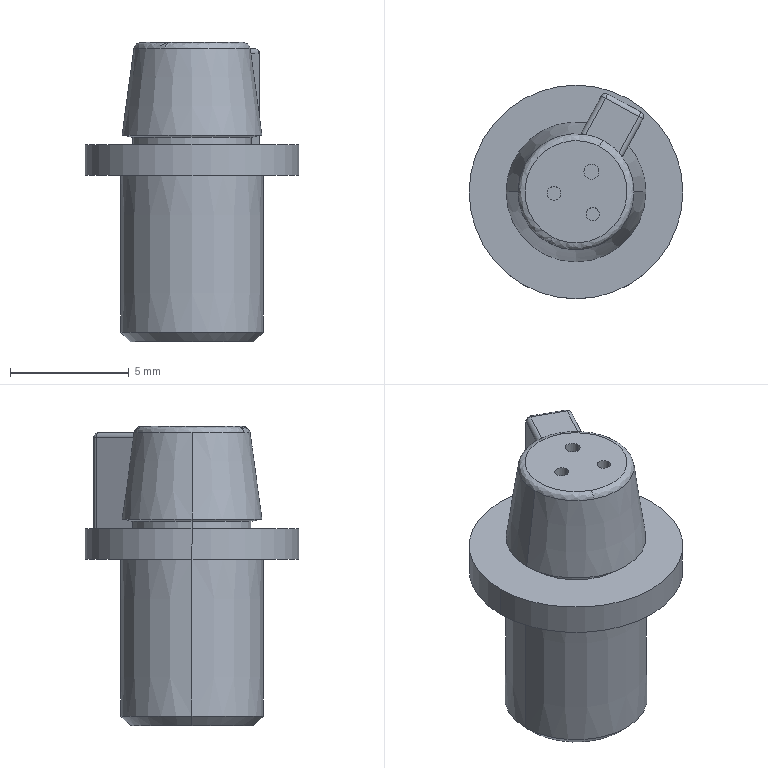Part | SolidWorks | features BaseBody 1 | 1 solid | 45 faces | box 9 x 9 x 12.6 mm | volume 296.292 mm3 | cylinder 19 | plane 12 | cone 10 | spline 4 | commonest cylinder face diameters 0.4 x6 5.005 x3 0.562 x2 0.587 x2 0.63 x2 4 x2
STEP:
#1=CARTESIAN_POINT('',(481.239,-70.69,314.885));
#2=VERTEX_POINT('',#1);
#3=CARTESIAN_POINT('',(480.554,-70.162,314.885));
#4=VERTEX_POINT('',#3);
#5=CARTESIAN_POINT('',(479.428,-72.334,314.885));
#6=DIRECTION('',(0.000000008,-0.000000005,1.));
#7=DIRECTION('',(-1.,0.,0.000000008));
#8=AXIS2_PLACEMENT_3D('',#5,#6,#7);
#9=CIRCLE('',#8,2.447);
#10=EDGE_CURVE('',#2,#4,#9,.T.);
#11=ORIENTED_EDGE('',*,*,#10,.T.);
#12=CARTESIAN_POINT('',(480.417,-70.426,315.144));
#13=VERTEX_POINT('',#12);
#14=CARTESIAN_POINT('',(480.417,-70.426,314.844));
#15=DIRECTION('',(0.8878,-0.4602,-0.000000009));
#16=DIRECTION('',(0.4602,0.8878,0.000000001));
#17=AXIS2_PLACEMENT_3D('',#14,#15,#16);
#18=CIRCLE('',#17,0.3);
#19=EDGE_CURVE('',#4,#13,#18,.T.);
#20=ORIENTED_EDGE('',*,*,#19,.T.);
#21=CARTESIAN_POINT('',(478.438,-74.243,315.144));
#22=VERTEX_POINT('',#21);
#23=CARTESIAN_POINT('',(480.417,-70.426,315.144));
#24=CARTESIAN_POINT('',(484.234,-72.404,315.144));
#25=CARTESIAN_POINT('',(482.255,-76.221,315.144));
#26=CARTESIAN_POINT('',(478.438,-74.243,315.144));
#27=(BOUNDED_CURVE()B_SPLINE_CURVE(3,(#23,#24,#25,#26),.UNSPECIFIED.,.F.,.F.)B_SPLINE_CURVE_WITH_KNOTS((4,4),(0.,1.),.UNSPECIFIED.)CURVE()GEOMETRIC_REPRESENTATION_ITEM()RATIONAL_B_SPLINE_CURVE((1.,0.3333,0.3333,1.))REPRESENTATION_ITEM(''));
#28=EDGE_CURVE('',#13,#22,#27,.T.);
#29=ORIENTED_EDGE('',*,*,#28,.T.);
#30=CARTESIAN_POINT('',(478.302,-74.506,314.885));
#31=VERTEX_POINT('',#30);
#32=CARTESIAN_POINT('',(478.438,-74.243,314.844));
#33=DIRECTION('',(-0.8878,0.4602,0.000000009));
#34=DIRECTION('',(-0.4602,-0.8878,-0.000000001));
#35=AXIS2_PLACEMENT_3D('',#32,#33,#34);
#36=CIRCLE('',#35,0.3);
#37=EDGE_CURVE('',#31,#22,#36,.T.);
#38=ORIENTED_EDGE('',*,*,#37,.F.);
#39=CARTESIAN_POINT('',(481.874,-72.334,314.885));
#40=VERTEX_POINT('',#39);
#41=CARTESIAN_POINT('',(479.428,-72.334,314.885));
#42=DIRECTION('',(-0.000000008,0.000000005,-1.));
#43=DIRECTION('',(0.4602,0.8878,0.000000001));
#44=AXIS2_PLACEMENT_3D('',#41,#42,#43);
#45=CIRCLE('',#44,2.447);
#46=EDGE_CURVE('',#40,#31,#45,.T.);
#47=ORIENTED_EDGE('',*,*,#46,.F.);
#48=CARTESIAN_POINT('',(479.428,-72.334,314.885));
#49=DIRECTION('',(-0.000000008,0.000000005,-1.));
#50=DIRECTION('',(0.4602,0.8878,0.000000001));
#51=AXIS2_PLACEMENT_3D('',#48,#49,#50);
#52=CIRCLE('',#51,2.447);
#53=EDGE_CURVE('',#2,#40,#52,.T.);
#54=ORIENTED_EDGE('',*,*,#53,.F.);
#55=EDGE_LOOP('',(#11,#20,#29,#38,#47,#54));
#56=FACE_OUTER_BOUND('',#55,.T.);
#57=CARTESIAN_POINT('',(480.554,-70.162,314.885));
#58=CARTESIAN_POINT('',(484.898,-72.414,314.885));
#59=CARTESIAN_POINT('',(482.646,-76.759,314.885));
#60=CARTESIAN_POINT('',(478.302,-74.506,314.885));
#61=CARTESIAN_POINT('',(480.544,-70.181,315.041));
#62=CARTESIAN_POINT('',(484.851,-72.413,315.041));
#63=CARTESIAN_POINT('',(482.618,-76.72,315.041));
#64=CARTESIAN_POINT('',(478.311,-74.487,315.041));
#65=CARTESIAN_POINT('',(480.489,-70.286,315.144));
#66=CARTESIAN_POINT('',(484.585,-72.41,315.144));
#67=CARTESIAN_POINT('',(482.462,-76.506,315.144));
#68=CARTESIAN_POINT('',(478.366,-74.382,315.144));
#69=CARTESIAN_POINT('',(480.417,-70.426,315.144));
#70=CARTESIAN_POINT('',(484.234,-72.404,315.144));
#71=CARTESIAN_POINT('',(482.255,-76.221,315.144));
#72=CARTESIAN_POINT('',(478.438,-74.243,315.144));
#73=(BOUNDED_SURFACE()B_SPLINE_SURFACE(3,3,((#57,#58,#59,#60),(#61,#62,#63,#64),(#65,#66,#67,#68),(#69,#70,#71,#72)),.UNSPECIFIED.,.F.,.F.,.F.)B_SPLINE_SURFACE_WITH_KNOTS((4,4),(4,4),(0.,1.),(0.,1.),.UNSPECIFIED.)GEOMETRIC_REPRESENTATION_ITEM()RATIONAL_B_SPLINE_SURFACE(((1.,0.3333,0.3333,1.),(0.8357,0.2786,0.2786,0.8357),(0.8357,0.2786,0.2786,0.8357),(1.,0.3333,0.3333,1.)))REPRESENTATION_ITEM('')SURFACE());
#74=ADVANCED_FACE('',(#56),#73,.T.);
#75=CARTESIAN_POINT('',(482.427,-72.334,302.944));
#76=VERTEX_POINT('',#75);
#77=CARTESIAN_POINT('',(476.429,-72.334,302.944));
#78=VERTEX_POINT('',#77);
#79=CARTESIAN_POINT('',(479.428,-72.334,302.944));
#80=DIRECTION('',(0.000000008,-0.000000005,1.));
#81=DIRECTION('',(0.8773,-0.4799,-0.000000009));
#82=AXIS2_PLACEMENT_3D('',#79,#80,#81);
#83=CIRCLE('',#82,2.999);
#84=EDGE_CURVE('',#76,#78,#83,.T.);
#85=ORIENTED_EDGE('',*,*,#84,.T.);
#86=CARTESIAN_POINT('',(476.428,-72.334,309.544));
#87=VERTEX_POINT('',#86);
#88=CARTESIAN_POINT('',(476.428,-72.334,309.544));
#89=DIRECTION('',(-0.0001745,-0.000000005,1.));
#90=VECTOR('',#89,1000.);
#91=LINE('',#88,#90);
#92=EDGE_CURVE('',#78,#87,#91,.T.);
#93=ORIENTED_EDGE('',*,*,#92,.T.);
#94=CARTESIAN_POINT('',(482.428,-72.334,309.544));
#95=VERTEX_POINT('',#94);
#96=CARTESIAN_POINT('',(479.428,-72.334,309.544));
#97=DIRECTION('',(-0.000000008,0.000000005,-1.));
#98=DIRECTION('',(1.,0.,-0.000000008));
#99=AXIS2_PLACEMENT_3D('',#96,#97,#98);
#100=CIRCLE('',#99,3.);
#101=EDGE_CURVE('',#87,#95,#100,.T.);
#102=ORIENTED_EDGE('',*,*,#101,.T.);
#103=CARTESIAN_POINT('',(482.428,-72.334,309.544));
#104=DIRECTION('',(0.0001745,-0.000000005,1.));
#105=VECTOR('',#104,1000.);
#106=LINE('',#103,#105);
#107=EDGE_CURVE('',#76,#95,#106,.T.);
#108=ORIENTED_EDGE('',*,*,#107,.F.);
#109=EDGE_LOOP('',(#85,#93,#102,#108));
#110=FACE_OUTER_BOUND('',#109,.T.);
#111=CARTESIAN_POINT('',(479.428,-72.334,309.544));
#112=DIRECTION('',(0.000000008,-0.000000005,1.));
#113=DIRECTION('',(1.,0.,-0.000000008));
#114=AXIS2_PLACEMENT_3D('',#111,#112,#113);
#115=CONICAL_SURFACE('',#114,3.,0.0001745);
#116=ADVANCED_FACE('',(#110),#115,.T.);
#117=CARTESIAN_POINT('',(482.026,-72.334,302.544));
#118=VERTEX_POINT('',#117);
#119=CARTESIAN_POINT('',(476.829,-72.334,302.544));
#120=VERTEX_POINT('',#119);
#121=CARTESIAN_POINT('',(479.428,-72.334,302.544));
#122=DIRECTION('',(0.000000008,-0.000000005,1.));
#123=DIRECTION('',(1.,0.,-0.000000008));
#124=AXIS2_PLACEMENT_3D('',#121,#122,#123);
#125=CIRCLE('',#124,2.599);
#126=EDGE_CURVE('',#118,#120,#125,.T.);
#127=ORIENTED_EDGE('',*,*,#126,.T.);
#128=CARTESIAN_POINT('',(476.429,-72.334,302.944));
#129=DIRECTION('',(-0.7072,-0.000000003,0.707));
#130=VECTOR('',#129,1000.);
#131=LINE('',#128,#130);
#132=EDGE_CURVE('',#120,#78,#131,.T.);
#133=ORIENTED_EDGE('',*,*,#132,.T.);
#134=ORIENTED_EDGE('',*,*,#84,.F.);
#135=CARTESIAN_POINT('',(482.427,-72.334,302.944));
#136=DIRECTION('',(0.7072,-0.000000003,0.707));
#137=VECTOR('',#136,1000.);
#138=LINE('',#135,#137);
#139=EDGE_CURVE('',#118,#76,#138,.T.);
#140=ORIENTED_EDGE('',*,*,#139,.F.);
#141=EDGE_LOOP('',(#127,#133,#134,#140));
#142=FACE_OUTER_BOUND('',#141,.T.);
#143=CARTESIAN_POINT('',(479.428,-72.334,302.944));
#144=DIRECTION('',(0.000000008,-0.000000005,1.));
#145=DIRECTION('',(1.,0.,-0.000000008));
#146=AXIS2_PLACEMENT_3D('',#143,#144,#145);
#147=CONICAL_SURFACE('',#146,2.999,0.7855);
#148=ADVANCED_FACE('',(#142),#147,.T.);
#149=CARTESIAN_POINT('',(474.928,-72.334,310.844));
#150=VERTEX_POINT('',#149);
#151=CARTESIAN_POINT('',(483.928,-72.334,310.844));
#152=VERTEX_POINT('',#151);
#153=CARTESIAN_POINT('',(479.428,-72.334,310.844));
#154=DIRECTION('',(-0.000000008,0.000000005,-1.));
#155=DIRECTION('',(-1.,0.,0.000000008));
#156=AXIS2_PLACEMENT_3D('',#153,#154,#155);
#157=CIRCLE('',#156,4.5);
#158=EDGE_CURVE('',#150,#152,#157,.T.);
#159=ORIENTED_EDGE('',*,*,#158,.T.);
#160=CARTESIAN_POINT('',(483.928,-72.334,309.544));
#161=VERTEX_POINT('',#160);
#162=CARTESIAN_POINT('',(483.928,-72.334,309.544));
#163=DIRECTION('',(-0.000000008,0.000000005,-1.));
#164=VECTOR('',#163,1000.);
#165=LINE('',#162,#164);
#166=EDGE_CURVE('',#152,#161,#165,.T.);
#167=ORIENTED_EDGE('',*,*,#166,.T.);
#168=CARTESIAN_POINT('',(474.928,-72.334,309.544));
#169=VERTEX_POINT('',#168);
#170=CARTESIAN_POINT('',(479.428,-72.334,309.544));
#171=DIRECTION('',(0.000000008,-0.000000005,1.));
#172=DIRECTION('',(-1.,0.,0.000000008));
#173=AXIS2_PLACEMENT_3D('',#170,#171,#172);
#174=CIRCLE('',#173,4.5);
#175=EDGE_CURVE('',#161,#169,#174,.T.);
#176=ORIENTED_EDGE('',*,*,#175,.T.);
#177=CARTESIAN_POINT('',(474.928,-72.334,309.544));
#178=DIRECTION('',(-0.000000008,0.000000005,-1.));
#179=VECTOR('',#178,1000.);
#180=LINE('',#177,#179);
#181=EDGE_CURVE('',#150,#169,#180,.T.);
#182=ORIENTED_EDGE('',*,*,#181,.F.);
#183=EDGE_LOOP('',(#159,#167,#176,#182));
#184=FACE_OUTER_BOUND('',#183,.T.);
#185=CARTESIAN_POINT('',(479.428,-72.334,309.544));
#186=DIRECTION('',(-0.000000008,0.000000005,-1.));
#187=DIRECTION('',(-1.,0.,0.000000008));
#188=AXIS2_PLACEMENT_3D('',#185,#186,#187);
#189=CYLINDRICAL_SURFACE('',#188,4.5);
#190=ADVANCED_FACE('',(#184),#189,.T.);
#191=CARTESIAN_POINT('',(481.428,-72.334,309.544));
#192=VERTEX_POINT('',#191);
#193=CARTESIAN_POINT('',(477.428,-72.334,309.544));
#194=VERTEX_POINT('',#193);
#195=CARTESIAN_POINT('',(479.428,-72.334,309.544));
#196=DIRECTION('',(-0.000000008,0.000000005,-1.));
#197=DIRECTION('',(-1.,0.,0.000000008));
#198=AXIS2_PLACEMENT_3D('',#195,#196,#197);
#199=CIRCLE('',#198,2.);
#200=EDGE_CURVE('',#192,#194,#199,.T.);
#201=ORIENTED_EDGE('',*,*,#200,.F.);
#202=CARTESIAN_POINT('',(481.428,-72.334,302.544));
#203=VERTEX_POINT('',#202);
#204=CARTESIAN_POINT('',(481.428,-72.334,302.544));
#205=DIRECTION('',(-0.000000008,0.000000005,-1.));
#206=VECTOR('',#205,1000.);
#207=LINE('',#204,#206);
#208=EDGE_CURVE('',#192,#203,#207,.T.);
#209=ORIENTED_EDGE('',*,*,#208,.T.);
#210=CARTESIAN_POINT('',(477.428,-72.334,302.544));
#211=VERTEX_POINT('',#210);
#212=CARTESIAN_POINT('',(479.428,-72.334,302.544));
#213=DIRECTION('',(0.000000008,-0.000000005,1.));
#214=DIRECTION('',(-1.,0.,0.000000008));
#215=AXIS2_PLACEMENT_3D('',#212,#213,#214);
#216=CIRCLE('',#215,2.);
#217=EDGE_CURVE('',#211,#203,#216,.T.);
#218=ORIENTED_EDGE('',*,*,#217,.F.);
#219=CARTESIAN_POINT('',(477.428,-72.334,302.544));
#220=DIRECTION('',(-0.000000008,0.000000005,-1.));
#221=VECTOR('',#220,1000.);
#222=LINE('',#219,#221);
#223=EDGE_CURVE('',#194,#211,#222,.T.);
#224=ORIENTED_EDGE('',*,*,#223,.F.);
#225=EDGE_LOOP('',(#201,#209,#218,#224));
#226=FACE_OUTER_BOUND('',#225,.T.);
#227=CARTESIAN_POINT('',(479.428,-72.334,302.544));
#228=DIRECTION('',(-0.000000008,0.000000005,-1.));
#229=DIRECTION('',(-1.,0.,0.000000008));
#230=AXIS2_PLACEMENT_3D('',#227,#228,#229);
#231=CYLINDRICAL_SURFACE('',#230,2.);
#232=ADVANCED_FACE('',(#226),#231,.F.);
#233=CARTESIAN_POINT('',(476.925,-72.334,310.844));
#234=VERTEX_POINT('',#233);
#235=CARTESIAN_POINT('',(479.652,-69.842,310.844));
#236=VERTEX_POINT('',#235);
#237=CARTESIAN_POINT('',(479.428,-72.334,310.844));
#238=DIRECTION('',(-0.000000008,0.000000005,-1.));
#239=DIRECTION('',(1.,0.,-0.000000008));
#240=AXIS2_PLACEMENT_3D('',#237,#238,#239);
#241=CIRCLE('',#240,2.503);
#242=EDGE_CURVE('',#234,#236,#241,.T.);
#243=ORIENTED_EDGE('',*,*,#242,.F.);
#244=CARTESIAN_POINT('',(476.925,-72.334,311.148));
#245=VERTEX_POINT('',#244);
#246=CARTESIAN_POINT('',(476.925,-72.334,310.996));
#247=DIRECTION('',(0.000000008,-0.000000005,1.));
#248=VECTOR('',#247,1000.);
#249=LINE('',#246,#248);
#250=EDGE_CURVE('',#234,#245,#249,.T.);
#251=ORIENTED_EDGE('',*,*,#250,.T.);
#252=CARTESIAN_POINT('',(479.652,-69.842,311.148));
#253=VERTEX_POINT('',#252);
#254=CARTESIAN_POINT('',(479.428,-72.334,311.148));
#255=DIRECTION('',(-0.000000008,0.000000005,-1.));
#256=DIRECTION('',(1.,0.,-0.000000008));
#257=AXIS2_PLACEMENT_3D('',#254,#255,#256);
#258=CIRCLE('',#257,2.503);
#259=EDGE_CURVE('',#245,#253,#258,.T.);
#260=ORIENTED_EDGE('',*,*,#259,.T.);
#261=CARTESIAN_POINT('',(479.652,-69.842,310.996));
#262=DIRECTION('',(-0.000000008,0.000000005,-1.));
#263=VECTOR('',#262,1000.);
#264=LINE('',#261,#263);
#265=EDGE_CURVE('',#253,#236,#264,.T.);
#266=ORIENTED_EDGE('',*,*,#265,.T.);
#267=EDGE_LOOP('',(#243,#251,#260,#266));
#268=FACE_OUTER_BOUND('',#267,.T.);
#269=CARTESIAN_POINT('',(479.428,-72.334,310.996));
#270=DIRECTION('',(0.000000008,-0.000000005,1.));
#271=DIRECTION('',(1.,0.,-0.000000008));
#272=AXIS2_PLACEMENT_3D('',#269,#270,#271);
#273=CYLINDRICAL_SURFACE('',#272,2.503);
#274=ADVANCED_FACE('',(#268),#273,.T.);
#275=ORIENTED_EDGE('',*,*,#250,.F.);
#276=CARTESIAN_POINT('',(481.93,-72.334,310.844));
#277=VERTEX_POINT('',#276);
#278=CARTESIAN_POINT('',(479.428,-72.334,310.844));
#279=DIRECTION('',(-0.000000008,0.000000005,-1.));
#280=DIRECTION('',(1.,0.,-0.000000008));
#281=AXIS2_PLACEMENT_3D('',#278,#279,#280);
#282=CIRCLE('',#281,2.503);
#283=EDGE_CURVE('',#277,#234,#282,.T.);
#284=ORIENTED_EDGE('',*,*,#283,.F.);
#285=CARTESIAN_POINT('',(481.93,-72.334,311.148));
#286=VERTEX_POINT('',#285);
#287=CARTESIAN_POINT('',(481.93,-72.334,310.996));
#288=DIRECTION('',(0.000000008,-0.000000005,1.));
#289=VECTOR('',#288,1000.);
#290=LINE('',#287,#289);
#291=EDGE_CURVE('',#277,#286,#290,.T.);
#292=ORIENTED_EDGE('',*,*,#291,.T.);
#293=CARTESIAN_POINT('',(479.428,-72.334,311.148));
#294=DIRECTION('',(-0.000000008,0.000000005,-1.));
#295=DIRECTION('',(1.,0.,-0.000000008));
#296=AXIS2_PLACEMENT_3D('',#293,#294,#295);
#297=CIRCLE('',#296,2.503);
#298=EDGE_CURVE('',#286,#245,#297,.T.);
#299=ORIENTED_EDGE('',*,*,#298,.T.);
#300=EDGE_LOOP('',(#275,#284,#292,#299));
#301=FACE_OUTER_BOUND('',#300,.T.);
#302=CARTESIAN_POINT('',(479.428,-72.334,310.996));
#303=DIRECTION('',(0.000000008,-0.000000005,1.));
#304=DIRECTION('',(1.,0.,-0.000000008));
#305=AXIS2_PLACEMENT_3D('',#302,#303,#304);
#306=CYLINDRICAL_SURFACE('',#305,2.503);
#307=ADVANCED_FACE('',(#301),#306,.T.);
#308=ORIENTED_EDGE('',*,*,#259,.F.);
#309=CARTESIAN_POINT('',(476.482,-72.334,311.244));
#310=VERTEX_POINT('',#309);
#311=CARTESIAN_POINT('',(476.482,-72.334,311.244));
#312=DIRECTION('',(-0.9773,-0.000000001,0.2119));
#313=VECTOR('',#312,1000.);
#314=LINE('',#311,#313);
#315=EDGE_CURVE('',#245,#310,#314,.T.);
#316=ORIENTED_EDGE('',*,*,#315,.T.);
#317=CARTESIAN_POINT('',(479.88,-69.424,311.244));
#318=VERTEX_POINT('',#317);
#319=CARTESIAN_POINT('',(479.428,-72.334,311.244));
#320=DIRECTION('',(-0.000000008,0.000000005,-1.));
#321=DIRECTION('',(0.4602,0.8878,0.000000001));
#322=AXIS2_PLACEMENT_3D('',#319,#320,#321);
#323=CIRCLE('',#322,2.945);
#324=EDGE_CURVE('',#310,#318,#323,.T.);
#325=ORIENTED_EDGE('',*,*,#324,.T.);
#326=CARTESIAN_POINT('',(479.652,-69.842,311.148));
#327=CARTESIAN_POINT('',(479.728,-69.702,311.179));
#328=CARTESIAN_POINT('',(479.804,-69.563,311.211));
#329=CARTESIAN_POINT('',(479.88,-69.424,311.244));
#330=B_SPLINE_CURVE_WITH_KNOTS('',3,(#326,#327,#328,#329),.UNSPECIFIED.,.F.,.F.,(4,4),(0.,0.0004857),.UNSPECIFIED.);
#331=EDGE_CURVE('',#253,#318,#330,.T.);
#332=ORIENTED_EDGE('',*,*,#331,.F.);
#333=EDGE_LOOP('',(#308,#316,#325,#332));
#334=FACE_OUTER_BOUND('',#333,.T.);
#335=CARTESIAN_POINT('',(479.428,-72.334,311.244));
#336=DIRECTION('',(0.000000008,-0.000000005,1.));
#337=DIRECTION('',(1.,0.,-0.000000008));
#338=AXIS2_PLACEMENT_3D('',#335,#336,#337);
#339=CONICAL_SURFACE('',#338,2.945,1.357);
#340=ADVANCED_FACE('',(#334),#339,.T.);
#341=ORIENTED_EDGE('',*,*,#315,.F.);
#342=ORIENTED_EDGE('',*,*,#298,.F.);
#343=CARTESIAN_POINT('',(482.373,-72.334,311.244));
#344=VERTEX_POINT('',#343);
#345=CARTESIAN_POINT('',(482.373,-72.334,311.244));
#346=DIRECTION('',(0.9773,-0.000000001,0.2119));
#347=VECTOR('',#346,1000.);
#348=LINE('',#345,#347);
#349=EDGE_CURVE('',#286,#344,#348,.T.);
#350=ORIENTED_EDGE('',*,*,#349,.T.);
#351=CARTESIAN_POINT('',(479.428,-72.334,311.244));
#352=DIRECTION('',(-0.000000008,0.000000005,-1.));
#353=DIRECTION('',(0.4602,0.8878,0.000000001));
#354=AXIS2_PLACEMENT_3D('',#351,#352,#353);
#355=CIRCLE('',#354,2.945);
#356=EDGE_CURVE('',#344,#310,#355,.T.);
#357=ORIENTED_EDGE('',*,*,#356,.T.);
#358=EDGE_LOOP('',(#341,#342,#350,#357));
#359=FACE_OUTER_BOUND('',#358,.T.);
#360=CARTESIAN_POINT('',(479.428,-72.334,311.244));
#361=DIRECTION('',(0.000000008,-0.000000005,1.));
#362=DIRECTION('',(1.,0.,-0.000000008));
#363=AXIS2_PLACEMENT_3D('',#360,#361,#362);
#364=CONICAL_SURFACE('',#363,2.945,1.357);
#365=ADVANCED_FACE('',(#359),#364,.T.);
#366=CARTESIAN_POINT('',(482.251,-69.257,310.844));
#367=VERTEX_POINT('',#366);
#368=CARTESIAN_POINT('',(482.276,-69.161,310.844));
#369=VERTEX_POINT('',#368);
#370=CARTESIAN_POINT('',(482.076,-69.161,310.844));
#371=DIRECTION('',(0.000000008,-0.000000005,1.));
#372=DIRECTION('',(1.,0.,-0.000000008));
#373=AXIS2_PLACEMENT_3D('',#370,#371,#372);
#374=CIRCLE('',#373,0.2);
#375=EDGE_CURVE('',#367,#369,#374,.T.);
#376=ORIENTED_EDGE('',*,*,#375,.T.);
#377=CARTESIAN_POINT('',(482.276,-69.161,314.685));
#378=VERTEX_POINT('',#377);
#379=CARTESIAN_POINT('',(482.276,-69.161,310.844));
#380=DIRECTION('',(0.000000008,-0.000000005,1.));
#381=VECTOR('',#380,1000.);
#382=LINE('',#379,#381);
#383=EDGE_CURVE('',#369,#378,#382,.T.);
#384=ORIENTED_EDGE('',*,*,#383,.T.);
#385=CARTESIAN_POINT('',(482.251,-69.257,314.685));
#386=VERTEX_POINT('',#385);
#387=CARTESIAN_POINT('',(482.076,-69.161,314.685));
#388=DIRECTION('',(-0.000000008,0.000000005,-1.));
#389=DIRECTION('',(1.,0.,-0.000000008));
#390=AXIS2_PLACEMENT_3D('',#387,#388,#389);
#391=CIRCLE('',#390,0.2);
#392=EDGE_CURVE('',#378,#386,#391,.T.);
#393=ORIENTED_EDGE('',*,*,#392,.T.);
#394=CARTESIAN_POINT('',(482.251,-69.257,310.844));
#395=DIRECTION('',(0.000000008,-0.000000004,1.));
#396=VECTOR('',#395,1000.);
#397=LINE('',#394,#396);
#398=EDGE_CURVE('',#367,#386,#397,.T.);
#399=ORIENTED_EDGE('',*,*,#398,.F.);
#400=EDGE_LOOP('',(#376,#384,#393,#399));
#401=FACE_OUTER_BOUND('',#400,.T.);
#402=CARTESIAN_POINT('',(482.076,-69.161,310.844));
#403=DIRECTION('',(0.000000008,-0.000000005,1.));
#404=DIRECTION('',(1.,0.,-0.000000008));
#405=AXIS2_PLACEMENT_3D('',#402,#403,#404);
#406=CYLINDRICAL_SURFACE('',#405,0.2);
#407=ADVANCED_FACE('',(#401),#406,.T.);
#408=ORIENTED_EDGE('',*,*,#53,.T.);
#409=CARTESIAN_POINT('',(482.373,-72.334,311.244));
#410=DIRECTION('',(0.1356,0.000000005,-0.9908));
#411=VECTOR('',#410,1000.);
#412=LINE('',#409,#411);
#413=EDGE_CURVE('',#40,#344,#412,.T.);
#414=ORIENTED_EDGE('',*,*,#413,.T.);
#415=CARTESIAN_POINT('',(481.635,-70.384,311.244));
#416=VERTEX_POINT('',#415);
#417=CARTESIAN_POINT('',(479.428,-72.334,311.244));
#418=DIRECTION('',(-0.000000008,0.000000005,-1.));
#419=DIRECTION('',(0.4602,0.8878,0.000000001));
#420=AXIS2_PLACEMENT_3D('',#417,#418,#419);
#421=CIRCLE('',#420,2.945);
#422=EDGE_CURVE('',#416,#344,#421,.T.);
#423=ORIENTED_EDGE('',*,*,#422,.F.);
#424=CARTESIAN_POINT('',(481.391,-70.829,314.685));
#425=VERTEX_POINT('',#424);
#426=CARTESIAN_POINT('',(481.391,-70.829,314.685));
#427=CARTESIAN_POINT('',(481.474,-70.678,313.538));
#428=CARTESIAN_POINT('',(481.555,-70.53,312.391));
#429=CARTESIAN_POINT('',(481.635,-70.384,311.244));
#430=B_SPLINE_CURVE_WITH_KNOTS('',3,(#426,#427,#428,#429),.UNSPECIFIED.,.F.,.F.,(4,4),(0.,0.003478),.UNSPECIFIED.);
#431=EDGE_CURVE('',#425,#416,#430,.T.);
#432=ORIENTED_EDGE('',*,*,#431,.F.);
#433=CARTESIAN_POINT('',(481.391,-70.829,314.685));
#434=CARTESIAN_POINT('',(481.387,-70.836,314.738));
#435=CARTESIAN_POINT('',(481.369,-70.823,314.792));
#436=CARTESIAN_POINT('',(481.312,-70.768,314.865));
#437=CARTESIAN_POINT('',(481.276,-70.73,314.885));
#438=CARTESIAN_POINT('',(481.239,-70.69,314.885));
#439=B_SPLINE_CURVE_WITH_KNOTS('',3,(#433,#434,#435,#436,#437,#438),.UNSPECIFIED.,.F.,.F.,(4,2,4),(0.,0.0001598,0.0003197),.UNSPECIFIED.);
#440=EDGE_CURVE('',#425,#2,#439,.T.);
#441=ORIENTED_EDGE('',*,*,#440,.T.);
#442=EDGE_LOOP('',(#408,#414,#423,#432,#441));
#443=FACE_OUTER_BOUND('',#442,.T.);
#444=CARTESIAN_POINT('',(479.428,-72.334,311.244));
#445=DIRECTION('',(-0.000000008,0.000000005,-1.));
#446=DIRECTION('',(-1.,0.,0.000000008));
#447=AXIS2_PLACEMENT_3D('',#444,#445,#446);
#448=CONICAL_SURFACE('',#447,2.945,0.1361);
#449=ADVANCED_FACE('',(#443),#448,.T.);
#450=ORIENTED_EDGE('',*,*,#413,.F.);
#451=ORIENTED_EDGE('',*,*,#46,.T.);
#452=CARTESIAN_POINT('',(476.981,-72.334,314.885));
#453=VERTEX_POINT('',#452);
#454=CARTESIAN_POINT('',(479.428,-72.334,314.885));
#455=DIRECTION('',(-0.000000008,0.000000005,-1.));
#456=DIRECTION('',(0.4602,0.8878,0.000000001));
#457=AXIS2_PLACEMENT_3D('',#454,#455,#456);
#458=CIRCLE('',#457,2.447);
#459=EDGE_CURVE('',#31,#453,#458,.T.);
#460=ORIENTED_EDGE('',*,*,#459,.T.);
#461=CARTESIAN_POINT('',(476.482,-72.334,311.244));
#462=DIRECTION('',(-0.1356,0.000000005,-0.9908));
#463=VECTOR('',#462,1000.);
#464=LINE('',#461,#463);
#465=EDGE_CURVE('',#453,#310,#464,.T.);
#466=ORIENTED_EDGE('',*,*,#465,.T.);
#467=ORIENTED_EDGE('',*,*,#356,.F.);
#468=EDGE_LOOP('',(#450,#451,#460,#466,#467));
#469=FACE_OUTER_BOUND('',#468,.T.);
#470=CARTESIAN_POINT('',(479.428,-72.334,311.244));
#471=DIRECTION('',(-0.000000008,0.000000005,-1.));
#472=DIRECTION('',(-1.,0.,0.000000008));
#473=AXIS2_PLACEMENT_3D('',#470,#471,#472);
#474=CONICAL_SURFACE('',#473,2.945,0.1361);
#475=ADVANCED_FACE('',(#469),#474,.T.);
#476=CARTESIAN_POINT('',(479.762,-71.484,310.144));
#477=VERTEX_POINT('',#476);
#478=CARTESIAN_POINT('',(480.392,-71.484,310.144));
#479=VERTEX_POINT('',#478);
#480=CARTESIAN_POINT('',(480.077,-71.484,310.144));
#481=DIRECTION('',(0.000000008,-0.000000005,1.));
#482=DIRECTION('',(1.,0.,-0.000000008));
#483=AXIS2_PLACEMENT_3D('',#480,#481,#482);
#484=CIRCLE('',#483,0.3151);
#485=EDGE_CURVE('',#477,#479,#484,.T.);
#486=ORIENTED_EDGE('',*,*,#485,.F.);
#487=CARTESIAN_POINT('',(479.762,-71.484,315.144));
#488=VERTEX_POINT('',#487);
#489=CARTESIAN_POINT('',(479.762,-71.484,315.144));
#490=DIRECTION('',(0.000000008,-0.000000005,1.));
#491=VECTOR('',#490,1000.);
#492=LINE('',#489,#491);
#493=EDGE_CURVE('',#477,#488,#492,.T.);
#494=ORIENTED_EDGE('',*,*,#493,.T.);
#495=CARTESIAN_POINT('',(480.392,-71.484,315.144));
#496=VERTEX_POINT('',#495);
#497=CARTESIAN_POINT('',(480.077,-71.484,315.144));
#498=DIRECTION('',(-0.000000008,0.000000005,-1.));
#499=DIRECTION('',(1.,0.,-0.000000008));
#500=AXIS2_PLACEMENT_3D('',#497,#498,#499);
#501=CIRCLE('',#500,0.3151);
#502=EDGE_CURVE('',#496,#488,#501,.T.);
#503=ORIENTED_EDGE('',*,*,#502,.F.);
#504=CARTESIAN_POINT('',(480.392,-71.484,315.144));
#505=DIRECTION('',(0.000000008,-0.000000005,1.));
#506=VECTOR('',#505,1000.);
#507=LINE('',#504,#506);
#508=EDGE_CURVE('',#479,#496,#507,.T.);
#509=ORIENTED_EDGE('',*,*,#508,.F.);
#510=EDGE_LOOP('',(#486,#494,#503,#509));
#511=FACE_OUTER_BOUND('',#510,.T.);
#512=CARTESIAN_POINT('',(480.077,-71.484,315.144));
#513=DIRECTION('',(0.000000008,-0.000000005,1.));
#514=DIRECTION('',(1.,0.,-0.000000008));
#515=AXIS2_PLACEMENT_3D('',#512,#513,#514);
#516=CYLINDRICAL_SURFACE('',#515,0.3151);
#517=ADVANCED_FACE('',(#511),#516,.F.);
#518=CARTESIAN_POINT('',(479.856,-73.279,310.144));
#519=VERTEX_POINT('',#518);
#520=CARTESIAN_POINT('',(480.418,-73.279,310.144));
#521=VERTEX_POINT('',#520);
#522=CARTESIAN_POINT('',(480.137,-73.279,310.144));
#523=DIRECTION('',(0.000000008,-0.000000005,1.));
#524=DIRECTION('',(1.,0.,-0.000000008));
#525=AXIS2_PLACEMENT_3D('',#522,#523,#524);
#526=CIRCLE('',#525,0.2808);
#527=EDGE_CURVE('',#519,#521,#526,.T.);
#528=ORIENTED_EDGE('',*,*,#527,.F.);
#529=CARTESIAN_POINT('',(479.856,-73.279,315.144));
#530=VERTEX_POINT('',#529);
#531=CARTESIAN_POINT('',(479.856,-73.279,315.144));
#532=DIRECTION('',(0.000000008,-0.000000005,1.));
#533=VECTOR('',#532,1000.);
#534=LINE('',#531,#533);
#535=EDGE_CURVE('',#519,#530,#534,.T.);
#536=ORIENTED_EDGE('',*,*,#535,.T.);
#537=CARTESIAN_POINT('',(480.418,-73.279,315.144));
#538=VERTEX_POINT('',#537);
#539=CARTESIAN_POINT('',(480.137,-73.279,315.144));
#540=DIRECTION('',(-0.000000008,0.000000005,-1.));
#541=DIRECTION('',(1.,0.,-0.000000008));
#542=AXIS2_PLACEMENT_3D('',#539,#540,#541);
#543=CIRCLE('',#542,0.2808);
#544=EDGE_CURVE('',#538,#530,#543,.T.);
#545=ORIENTED_EDGE('',*,*,#544,.F.);
#546=CARTESIAN_POINT('',(480.418,-73.279,315.144));
#547=DIRECTION('',(0.000000008,-0.000000005,1.));
#548=VECTOR('',#547,1000.);
#549=LINE('',#546,#548);
#550=EDGE_CURVE('',#521,#538,#549,.T.);
#551=ORIENTED_EDGE('',*,*,#550,.F.);
#552=EDGE_LOOP('',(#528,#536,#545,#551));
#553=FACE_OUTER_BOUND('',#552,.T.);
#554=CARTESIAN_POINT('',(480.137,-73.279,315.144));
#555=DIRECTION('',(0.000000008,-0.000000005,1.));
#556=DIRECTION('',(1.,0.,-0.000000008));
#557=AXIS2_PLACEMENT_3D('',#554,#555,#556);
#558=CYLINDRICAL_SURFACE('',#557,0.2808);
#559=ADVANCED_FACE('',(#553),#558,.F.);
#560=CARTESIAN_POINT('',(478.209,-72.4,310.144));
#561=VERTEX_POINT('',#560);
#562=CARTESIAN_POINT('',(478.795,-72.4,310.144));
#563=VERTEX_POINT('',#562);
#564=CARTESIAN_POINT('',(478.502,-72.4,310.144));
#565=DIRECTION('',(0.000000008,-0.000000005,1.));
#566=DIRECTION('',(1.,0.,-0.000000008));
#567=AXIS2_PLACEMENT_3D('',#564,#565,#566);
#568=CIRCLE('',#567,0.2933);
#569=EDGE_CURVE('',#561,#563,#568,.T.);
#570=ORIENTED_EDGE('',*,*,#569,.F.);
#571=CARTESIAN_POINT('',(478.209,-72.4,315.144));
#572=VERTEX_POINT('',#571);
#573=CARTESIAN_POINT('',(478.209,-72.4,315.144));
#574=DIRECTION('',(0.000000008,-0.000000005,1.));
#575=VECTOR('',#574,1000.);
#576=LINE('',#573,#575);
#577=EDGE_CURVE('',#561,#572,#576,.T.);
#578=ORIENTED_EDGE('',*,*,#577,.T.);
#579=CARTESIAN_POINT('',(478.795,-72.4,315.144));
#580=VERTEX_POINT('',#579);
#581=CARTESIAN_POINT('',(478.502,-72.4,315.144));
#582=DIRECTION('',(-0.000000008,0.000000005,-1.));
#583=DIRECTION('',(1.,0.,-0.000000008));
#584=AXIS2_PLACEMENT_3D('',#581,#582,#583);
#585=CIRCLE('',#584,0.2933);
#586=EDGE_CURVE('',#580,#572,#585,.T.);
#587=ORIENTED_EDGE('',*,*,#586,.F.);
#588=CARTESIAN_POINT('',(478.795,-72.4,315.144));
#589=DIRECTION('',(0.000000008,-0.000000005,1.));
#590=VECTOR('',#589,1000.);
#591=LINE('',#588,#590);
#592=EDGE_CURVE('',#563,#580,#591,.T.);
#593=ORIENTED_EDGE('',*,*,#592,.F.);
#594=EDGE_LOOP('',(#570,#578,#587,#593));
#595=FACE_OUTER_BOUND('',#594,.T.);
#596=CARTESIAN_POINT('',(478.502,-72.4,315.144));
#597=DIRECTION('',(0.000000008,-0.000000005,1.));
#598=DIRECTION('',(1.,0.,-0.000000008));
#599=AXIS2_PLACEMENT_3D('',#596,#597,#598);
#600=CYLINDRICAL_SURFACE('',#599,0.2933);
#601=ADVANCED_FACE('',(#595),#600,.F.);
#602=ORIENTED_EDGE('',*,*,#92,.F.);
#603=CARTESIAN_POINT('',(479.428,-72.334,302.944));
#604=DIRECTION('',(0.000000008,-0.000000005,1.));
#605=DIRECTION('',(0.8773,-0.4799,-0.000000009));
#606=AXIS2_PLACEMENT_3D('',#603,#604,#605);
#607=CIRCLE('',#606,2.999);
#608=EDGE_CURVE('',#78,#76,#607,.T.);
#609=ORIENTED_EDGE('',*,*,#608,.T.);
#610=ORIENTED_EDGE('',*,*,#107,.T.);
#611=CARTESIAN_POINT('',(479.428,-72.334,309.544));
#612=DIRECTION('',(-0.000000008,0.000000005,-1.));
#613=DIRECTION('',(1.,0.,-0.000000008));
#614=AXIS2_PLACEMENT_3D('',#611,#612,#613);
#615=CIRCLE('',#614,3.);
#616=EDGE_CURVE('',#95,#87,#615,.T.);
#617=ORIENTED_EDGE('',*,*,#616,.T.);
#618=EDGE_LOOP('',(#602,#609,#610,#617));
#619=FACE_OUTER_BOUND('',#618,.T.);
#620=CARTESIAN_POINT('',(479.428,-72.334,309.544));
#621=DIRECTION('',(0.000000008,-0.000000005,1.));
#622=DIRECTION('',(1.,0.,-0.000000008));
#623=AXIS2_PLACEMENT_3D('',#620,#621,#622);
#624=CONICAL_SURFACE('',#623,3.,0.0001745);
#625=ADVANCED_FACE('',(#619),#624,.T.);
#626=ORIENTED_EDGE('',*,*,#132,.F.);
#627=CARTESIAN_POINT('',(479.428,-72.334,302.544));
#628=DIRECTION('',(0.000000008,-0.000000005,1.));
#629=DIRECTION('',(1.,0.,-0.000000008));
#630=AXIS2_PLACEMENT_3D('',#627,#628,#629);
#631=CIRCLE('',#630,2.599);
#632=EDGE_CURVE('',#120,#118,#631,.T.);
#633=ORIENTED_EDGE('',*,*,#632,.T.);
#634=ORIENTED_EDGE('',*,*,#139,.T.);
#635=ORIENTED_EDGE('',*,*,#608,.F.);
#636=EDGE_LOOP('',(#626,#633,#634,#635));
#637=FACE_OUTER_BOUND('',#636,.T.);
#638=CARTESIAN_POINT('',(479.428,-72.334,302.944));
#639=DIRECTION('',(0.000000008,-0.000000005,1.));
#640=DIRECTION('',(1.,0.,-0.000000008));
#641=AXIS2_PLACEMENT_3D('',#638,#639,#640);
#642=CONICAL_SURFACE('',#641,2.999,0.7855);
#643=ADVANCED_FACE('',(#637),#642,.T.);
#644=CARTESIAN_POINT('',(479.428,-72.334,309.544));
#645=DIRECTION('',(0.000000008,-0.000000005,1.));
#646=DIRECTION('',(-1.,0.,0.000000008));
#647=AXIS2_PLACEMENT_3D('',#644,#645,#646);
#648=CIRCLE('',#647,4.5);
#649=EDGE_CURVE('',#169,#161,#648,.T.);
#650=ORIENTED_EDGE('',*,*,#649,.F.);
#651=ORIENTED_EDGE('',*,*,#175,.F.);
#652=EDGE_LOOP('',(#650,#651));
#653=FACE_OUTER_BOUND('',#652,.T.);
#654=ORIENTED_EDGE('',*,*,#616,.F.);
#655=ORIENTED_EDGE('',*,*,#101,.F.);
#656=EDGE_LOOP('',(#654,#655));
#657=FACE_BOUND('',#656,.T.);
#658=CARTESIAN_POINT('',(479.428,-72.334,309.544));
#659=DIRECTION('',(0.000000008,-0.000000005,1.));
#660=DIRECTION('',(1.,0.,-0.000000008));
#661=AXIS2_PLACEMENT_3D('',#658,#659,#660);
#662=PLANE('',#661);
#663=ADVANCED_FACE('',(#653,#657),#662,.F.);
#664=ORIENTED_EDGE('',*,*,#126,.F.);
#665=ORIENTED_EDGE('',*,*,#632,.F.);
#666=EDGE_LOOP('',(#664,#665));
#667=FACE_OUTER_BOUND('',#666,.T.);
#668=ORIENTED_EDGE('',*,*,#217,.T.);
#669=CARTESIAN_POINT('',(479.428,-72.334,302.544));
#670=DIRECTION('',(0.000000008,-0.000000005,1.));
#671=DIRECTION('',(-1.,0.,0.000000008));
#672=AXIS2_PLACEMENT_3D('',#669,#670,#671);
#673=CIRCLE('',#672,2.);
#674=EDGE_CURVE('',#203,#211,#673,.T.);
#675=ORIENTED_EDGE('',*,*,#674,.T.);
#676=EDGE_LOOP('',(#668,#675));
#677=FACE_BOUND('',#676,.T.);
#678=CARTESIAN_POINT('',(479.428,-72.334,302.544));
#679=DIRECTION('',(-0.000000008,0.000000005,-1.));
#680=DIRECTION('',(-1.,0.,0.000000008));
#681=AXIS2_PLACEMENT_3D('',#678,#679,#680);
#682=PLANE('',#681);
#683=ADVANCED_FACE('',(#667,#677),#682,.T.);
#684=ORIENTED_EDGE('',*,*,#166,.F.);
#685=CARTESIAN_POINT('',(479.428,-72.334,310.844));
#686=DIRECTION('',(-0.000000008,0.000000005,-1.));
#687=DIRECTION('',(-1.,0.,0.000000008));
#688=AXIS2_PLACEMENT_3D('',#685,#686,#687);
#689=CIRCLE('',#688,4.5);
#690=EDGE_CURVE('',#152,#150,#689,.T.);
#691=ORIENTED_EDGE('',*,*,#690,.T.);
#692=ORIENTED_EDGE('',*,*,#181,.T.);
#693=ORIENTED_EDGE('',*,*,#649,.T.);
#694=EDGE_LOOP('',(#684,#691,#692,#693));
#695=FACE_OUTER_BOUND('',#694,.T.);
#696=CARTESIAN_POINT('',(479.428,-72.334,309.544));
#697=DIRECTION('',(-0.000000008,0.000000005,-1.));
#698=DIRECTION('',(-1.,0.,0.000000008));
#699=AXIS2_PLACEMENT_3D('',#696,#697,#698);
#700=CYLINDRICAL_SURFACE('',#699,4.5);
#701=ADVANCED_FACE('',(#695),#700,.T.);
#702=ORIENTED_EDGE('',*,*,#208,.F.);
#703=CARTESIAN_POINT('',(479.428,-72.334,309.544));
#704=DIRECTION('',(-0.000000008,0.000000005,-1.));
#705=DIRECTION('',(-1.,0.,0.000000008));
#706=AXIS2_PLACEMENT_3D('',#703,#704,#705);
#707=CIRCLE('',#706,2.);
#708=EDGE_CURVE('',#194,#192,#707,.T.);
#709=ORIENTED_EDGE('',*,*,#708,.F.);
#710=ORIENTED_EDGE('',*,*,#223,.T.);
#711=ORIENTED_EDGE('',*,*,#674,.F.);
#712=EDGE_LOOP('',(#702,#709,#710,#711));
#713=FACE_OUTER_BOUND('',#712,.T.);
#714=CARTESIAN_POINT('',(479.428,-72.334,302.544));
#715=DIRECTION('',(-0.000000008,0.000000005,-1.));
#716=DIRECTION('',(-1.,0.,0.000000008));
#717=AXIS2_PLACEMENT_3D('',#714,#715,#716);
#718=CYLINDRICAL_SURFACE('',#717,2.);
#719=ADVANCED_FACE('',(#713),#718,.F.);
#720=CARTESIAN_POINT('',(481.406,-70.802,310.844));
#721=VERTEX_POINT('',#720);
#722=CARTESIAN_POINT('',(482.251,-69.257,310.844));
#723=DIRECTION('',(-0.4799,-0.8773,0.));
#724=VECTOR('',#723,1000.);
#725=LINE('',#722,#724);
#726=EDGE_CURVE('',#367,#721,#725,.T.);
#727=ORIENTED_EDGE('',*,*,#726,.T.);
#728=CARTESIAN_POINT('',(479.428,-72.334,310.844));
#729=DIRECTION('',(-0.000000008,0.000000005,-1.));
#730=DIRECTION('',(1.,0.,-0.000000008));
#731=AXIS2_PLACEMENT_3D('',#728,#729,#730);
#732=CIRCLE('',#731,2.503);
#733=EDGE_CURVE('',#721,#277,#732,.T.);
#734=ORIENTED_EDGE('',*,*,#733,.T.);
#735=ORIENTED_EDGE('',*,*,#283,.T.);
#736=ORIENTED_EDGE('',*,*,#242,.T.);
#737=CARTESIAN_POINT('',(480.497,-68.297,310.844));
#738=VERTEX_POINT('',#737);
#739=CARTESIAN_POINT('',(479.652,-69.842,310.844));
#740=DIRECTION('',(0.4799,0.8773,0.));
#741=VECTOR('',#740,1000.);
#742=LINE('',#739,#741);
#743=EDGE_CURVE('',#236,#738,#742,.T.);
#744=ORIENTED_EDGE('',*,*,#743,.T.);
#745=CARTESIAN_POINT('',(480.768,-68.217,310.844));
#746=VERTEX_POINT('',#745);
#747=CARTESIAN_POINT('',(480.672,-68.393,310.844));
#748=DIRECTION('',(0.000000008,-0.000000005,1.));
#749=DIRECTION('',(1.,0.,-0.000000008));
#750=AXIS2_PLACEMENT_3D('',#747,#748,#749);
#751=CIRCLE('',#750,0.2);
#752=EDGE_CURVE('',#746,#738,#751,.T.);
#753=ORIENTED_EDGE('',*,*,#752,.F.);
#754=CARTESIAN_POINT('',(482.172,-68.985,310.844));
#755=VERTEX_POINT('',#754);
#756=CARTESIAN_POINT('',(480.593,-68.121,310.844));
#757=DIRECTION('',(-0.8773,0.4799,0.));
#758=VECTOR('',#757,1000.);
#759=LINE('',#756,#758);
#760=EDGE_CURVE('',#755,#746,#759,.T.);
#761=ORIENTED_EDGE('',*,*,#760,.F.);
#762=CARTESIAN_POINT('',(482.076,-69.161,310.844));
#763=DIRECTION('',(0.000000008,-0.000000005,1.));
#764=DIRECTION('',(1.,0.,-0.000000008));
#765=AXIS2_PLACEMENT_3D('',#762,#763,#764);
#766=CIRCLE('',#765,0.2);
#767=EDGE_CURVE('',#369,#755,#766,.T.);
#768=ORIENTED_EDGE('',*,*,#767,.F.);
#769=ORIENTED_EDGE('',*,*,#375,.F.);
#770=EDGE_LOOP('',(#727,#734,#735,#736,#744,#753,#761,#768,#769));
#771=FACE_BOUND('',#770,.T.);
#772=ORIENTED_EDGE('',*,*,#158,.F.);
#773=ORIENTED_EDGE('',*,*,#690,.F.);
#774=EDGE_LOOP('',(#772,#773));
#775=FACE_OUTER_BOUND('',#774,.T.);
#776=CARTESIAN_POINT('',(479.428,-72.334,310.844));
#777=DIRECTION('',(0.000000008,-0.000000005,1.));
#778=DIRECTION('',(1.,0.,-0.000000008));
#779=AXIS2_PLACEMENT_3D('',#776,#777,#778);
#780=PLANE('',#779);
#781=ADVANCED_FACE('',(#771,#775),#780,.T.);
#782=ORIENTED_EDGE('',*,*,#708,.T.);
#783=ORIENTED_EDGE('',*,*,#200,.T.);
#784=EDGE_LOOP('',(#782,#783));
#785=FACE_OUTER_BOUND('',#784,.T.);
#786=CARTESIAN_POINT('',(479.428,-72.334,309.544));
#787=DIRECTION('',(0.000000008,-0.000000005,1.));
#788=DIRECTION('',(1.,0.,-0.000000008));
#789=AXIS2_PLACEMENT_3D('',#786,#787,#788);
#790=PLANE('',#789);
#791=ADVANCED_FACE('',(#785),#790,.F.);
#792=ORIENTED_EDGE('',*,*,#291,.F.);
#793=ORIENTED_EDGE('',*,*,#733,.F.);
#794=CARTESIAN_POINT('',(481.406,-70.802,311.148));
#795=VERTEX_POINT('',#794);
#796=CARTESIAN_POINT('',(481.406,-70.802,310.996));
#797=DIRECTION('',(0.000000008,-0.000000005,1.));
#798=VECTOR('',#797,1000.);
#799=LINE('',#796,#798);
#800=EDGE_CURVE('',#721,#795,#799,.T.);
#801=ORIENTED_EDGE('',*,*,#800,.T.);
#802=CARTESIAN_POINT('',(479.428,-72.334,311.148));
#803=DIRECTION('',(-0.000000008,0.000000005,-1.));
#804=DIRECTION('',(1.,0.,-0.000000008));
#805=AXIS2_PLACEMENT_3D('',#802,#803,#804);
#806=CIRCLE('',#805,2.503);
#807=EDGE_CURVE('',#795,#286,#806,.T.);
#808=ORIENTED_EDGE('',*,*,#807,.T.);
#809=EDGE_LOOP('',(#792,#793,#801,#808));
#810=FACE_OUTER_BOUND('',#809,.T.);
#811=CARTESIAN_POINT('',(479.428,-72.334,310.996));
#812=DIRECTION('',(0.000000008,-0.000000005,1.));
#813=DIRECTION('',(1.,0.,-0.000000008));
#814=AXIS2_PLACEMENT_3D('',#811,#812,#813);
#815=CYLINDRICAL_SURFACE('',#814,2.503);
#816=ADVANCED_FACE('',(#810),#815,.T.);
#817=ORIENTED_EDGE('',*,*,#726,.F.);
#818=ORIENTED_EDGE('',*,*,#398,.T.);
#819=CARTESIAN_POINT('',(482.347,-69.081,314.685));
#820=DIRECTION('',(-0.4799,-0.8773,0.));
#821=VECTOR('',#820,1000.);
#822=LINE('',#819,#821);
#823=EDGE_CURVE('',#386,#425,#822,.T.);
#824=ORIENTED_EDGE('',*,*,#823,.T.);
#825=ORIENTED_EDGE('',*,*,#431,.T.);
#826=CARTESIAN_POINT('',(481.635,-70.384,311.244));
#827=CARTESIAN_POINT('',(481.559,-70.523,311.211));
#828=CARTESIAN_POINT('',(481.482,-70.662,311.179));
#829=CARTESIAN_POINT('',(481.406,-70.802,311.148));
#830=B_SPLINE_CURVE_WITH_KNOTS('',3,(#826,#827,#828,#829),.UNSPECIFIED.,.F.,.F.,(4,4),(0.,0.0004857),.UNSPECIFIED.);
#831=EDGE_CURVE('',#416,#795,#830,.T.);
#832=ORIENTED_EDGE('',*,*,#831,.T.);
#833=ORIENTED_EDGE('',*,*,#800,.F.);
#834=EDGE_LOOP('',(#817,#818,#824,#825,#832,#833));
#835=FACE_OUTER_BOUND('',#834,.T.);
#836=CARTESIAN_POINT('',(482.347,-69.081,310.844));
#837=DIRECTION('',(0.8773,-0.4799,-0.000000009));
#838=DIRECTION('',(0.4799,0.8773,0.));
#839=AXIS2_PLACEMENT_3D('',#836,#837,#838);
#840=PLANE('',#839);
#841=ADVANCED_FACE('',(#835),#840,.T.);
#842=ORIENTED_EDGE('',*,*,#331,.T.);
#843=CARTESIAN_POINT('',(479.637,-69.869,314.685));
#844=VERTEX_POINT('',#843);
#845=CARTESIAN_POINT('',(479.88,-69.424,311.244));
#846=CARTESIAN_POINT('',(479.8,-69.57,312.391));
#847=CARTESIAN_POINT('',(479.719,-69.718,313.538));
#848=CARTESIAN_POINT('',(479.637,-69.869,314.685));
#849=B_SPLINE_CURVE_WITH_KNOTS('',3,(#845,#846,#847,#848),.UNSPECIFIED.,.F.,.F.,(4,4),(0.,0.003478),.UNSPECIFIED.);
#850=EDGE_CURVE('',#318,#844,#849,.T.);
#851=ORIENTED_EDGE('',*,*,#850,.T.);
#852=CARTESIAN_POINT('',(480.497,-68.297,314.685));
#853=VERTEX_POINT('',#852);
#854=CARTESIAN_POINT('',(479.537,-70.052,314.685));
#855=DIRECTION('',(0.4799,0.8773,0.));
#856=VECTOR('',#855,1000.);
#857=LINE('',#854,#856);
#858=EDGE_CURVE('',#844,#853,#857,.T.);
#859=ORIENTED_EDGE('',*,*,#858,.T.);
#860=CARTESIAN_POINT('',(480.497,-68.297,310.844));
#861=DIRECTION('',(-0.000000008,0.000000004,-1.));
#862=VECTOR('',#861,1000.);
#863=LINE('',#860,#862);
#864=EDGE_CURVE('',#853,#738,#863,.T.);
#865=ORIENTED_EDGE('',*,*,#864,.T.);
#866=ORIENTED_EDGE('',*,*,#743,.F.);
#867=ORIENTED_EDGE('',*,*,#265,.F.);
#868=EDGE_LOOP('',(#842,#851,#859,#865,#866,#867));
#869=FACE_OUTER_BOUND('',#868,.T.);
#870=CARTESIAN_POINT('',(479.537,-70.052,310.844));
#871=DIRECTION('',(-0.8773,0.4799,0.000000009));
#872=DIRECTION('',(-0.4799,-0.8773,0.));
#873=AXIS2_PLACEMENT_3D('',#870,#871,#872);
#874=PLANE('',#873);
#875=ADVANCED_FACE('',(#869),#874,.T.);
#876=ORIENTED_EDGE('',*,*,#349,.F.);
#877=ORIENTED_EDGE('',*,*,#807,.F.);
#878=ORIENTED_EDGE('',*,*,#831,.F.);
#879=ORIENTED_EDGE('',*,*,#422,.T.);
#880=EDGE_LOOP('',(#876,#877,#878,#879));
#881=FACE_OUTER_BOUND('',#880,.T.);
#882=CARTESIAN_POINT('',(479.428,-72.334,311.244));
#883=DIRECTION('',(0.000000008,-0.000000005,1.));
#884=DIRECTION('',(1.,0.,-0.000000008));
#885=AXIS2_PLACEMENT_3D('',#882,#883,#884);
#886=CONICAL_SURFACE('',#885,2.945,1.357);
#887=ADVANCED_FACE('',(#881),#886,.T.);
#888=ORIENTED_EDGE('',*,*,#383,.F.);
#889=ORIENTED_EDGE('',*,*,#767,.T.);
#890=CARTESIAN_POINT('',(482.172,-68.985,314.685));
#891=VERTEX_POINT('',#890);
#892=CARTESIAN_POINT('',(482.172,-68.985,310.844));
#893=DIRECTION('',(0.000000008,-0.000000005,1.));
#894=VECTOR('',#893,1000.);
#895=LINE('',#892,#894);
#896=EDGE_CURVE('',#755,#891,#895,.T.);
#897=ORIENTED_EDGE('',*,*,#896,.T.);
#898=CARTESIAN_POINT('',(482.076,-69.161,314.685));
#899=DIRECTION('',(-0.000000008,0.000000005,-1.));
#900=DIRECTION('',(1.,0.,-0.000000008));
#901=AXIS2_PLACEMENT_3D('',#898,#899,#900);
#902=CIRCLE('',#901,0.2);
#903=EDGE_CURVE('',#891,#378,#902,.T.);
#904=ORIENTED_EDGE('',*,*,#903,.T.);
#905=EDGE_LOOP('',(#888,#889,#897,#904));
#906=FACE_OUTER_BOUND('',#905,.T.);
#907=CARTESIAN_POINT('',(482.076,-69.161,310.844));
#908=DIRECTION('',(0.000000008,-0.000000005,1.));
#909=DIRECTION('',(1.,0.,-0.000000008));
#910=AXIS2_PLACEMENT_3D('',#907,#908,#909);
#911=CYLINDRICAL_SURFACE('',#910,0.2);
#912=ADVANCED_FACE('',(#906),#911,.T.);
#913=ORIENTED_EDGE('',*,*,#465,.F.);
#914=CARTESIAN_POINT('',(479.836,-69.922,314.885));
#915=VERTEX_POINT('',#914);
#916=CARTESIAN_POINT('',(479.428,-72.334,314.885));
#917=DIRECTION('',(-0.000000008,0.000000005,-1.));
#918=DIRECTION('',(0.4602,0.8878,0.000000001));
#919=AXIS2_PLACEMENT_3D('',#916,#917,#918);
#920=CIRCLE('',#919,2.447);
#921=EDGE_CURVE('',#453,#915,#920,.T.);
#922=ORIENTED_EDGE('',*,*,#921,.T.);
#923=CARTESIAN_POINT('',(479.836,-69.922,314.885));
#924=CARTESIAN_POINT('',(479.783,-69.913,314.885));
#925=CARTESIAN_POINT('',(479.73,-69.903,314.865));
#926=CARTESIAN_POINT('',(479.654,-69.885,314.792));
#927=CARTESIAN_POINT('',(479.633,-69.876,314.738));
#928=CARTESIAN_POINT('',(479.637,-69.869,314.685));
#929=B_SPLINE_CURVE_WITH_KNOTS('',3,(#923,#924,#925,#926,#927,#928),.UNSPECIFIED.,.F.,.F.,(4,2,4),(-0.000163,-0.000002991,0.000157),.UNSPECIFIED.);
#930=EDGE_CURVE('',#915,#844,#929,.T.);
#931=ORIENTED_EDGE('',*,*,#930,.T.);
#932=ORIENTED_EDGE('',*,*,#850,.F.);
#933=ORIENTED_EDGE('',*,*,#324,.F.);
#934=EDGE_LOOP('',(#913,#922,#931,#932,#933));
#935=FACE_OUTER_BOUND('',#934,.T.);
#936=CARTESIAN_POINT('',(479.428,-72.334,311.244));
#937=DIRECTION('',(-0.000000008,0.000000005,-1.));
#938=DIRECTION('',(-1.,0.,0.000000008));
#939=AXIS2_PLACEMENT_3D('',#936,#937,#938);
#940=CONICAL_SURFACE('',#939,2.945,0.1361);
#941=ADVANCED_FACE('',(#935),#940,.T.);
#942=ORIENTED_EDGE('',*,*,#823,.F.);
#943=CARTESIAN_POINT('',(482.076,-69.161,314.885));
#944=VERTEX_POINT('',#943);
#945=CARTESIAN_POINT('',(482.076,-69.161,314.685));
#946=DIRECTION('',(-0.4799,-0.8773,0.));
#947=DIRECTION('',(0.8773,-0.4799,0.));
#948=AXIS2_PLACEMENT_3D('',#945,#946,#947);
#949=CIRCLE('',#948,0.2);
#950=EDGE_CURVE('',#386,#944,#949,.T.);
#951=ORIENTED_EDGE('',*,*,#950,.T.);
#952=CARTESIAN_POINT('',(481.908,-69.468,314.885));
#953=DIRECTION('',(-0.4799,-0.8773,0.));
#954=VECTOR('',#953,1000.);
#955=LINE('',#952,#954);
#956=EDGE_CURVE('',#944,#2,#955,.T.);
#957=ORIENTED_EDGE('',*,*,#956,.T.);
#958=ORIENTED_EDGE('',*,*,#440,.F.);
#959=EDGE_LOOP('',(#942,#951,#957,#958));
#960=FACE_OUTER_BOUND('',#959,.T.);
#961=CARTESIAN_POINT('',(481.908,-69.468,314.685));
#962=DIRECTION('',(-0.4799,-0.8773,0.));
#963=DIRECTION('',(0.8773,-0.4799,0.));
#964=AXIS2_PLACEMENT_3D('',#961,#962,#963);
#965=CYLINDRICAL_SURFACE('',#964,0.2);
#966=ADVANCED_FACE('',(#960),#965,.T.);
#967=ORIENTED_EDGE('',*,*,#864,.F.);
#968=CARTESIAN_POINT('',(480.768,-68.217,314.685));
#969=VERTEX_POINT('',#968);
#970=CARTESIAN_POINT('',(480.672,-68.393,314.685));
#971=DIRECTION('',(-0.000000008,0.000000005,-1.));
#972=DIRECTION('',(1.,0.,-0.000000008));
#973=AXIS2_PLACEMENT_3D('',#970,#971,#972);
#974=CIRCLE('',#973,0.2);
#975=EDGE_CURVE('',#853,#969,#974,.T.);
#976=ORIENTED_EDGE('',*,*,#975,.T.);
#977=CARTESIAN_POINT('',(480.768,-68.217,310.844));
#978=DIRECTION('',(-0.000000008,0.000000005,-1.));
#979=VECTOR('',#978,1000.);
#980=LINE('',#977,#979);
#981=EDGE_CURVE('',#969,#746,#980,.T.);
#982=ORIENTED_EDGE('',*,*,#981,.T.);
#983=ORIENTED_EDGE('',*,*,#752,.T.);
#984=EDGE_LOOP('',(#967,#976,#982,#983));
#985=FACE_OUTER_BOUND('',#984,.T.);
#986=CARTESIAN_POINT('',(480.672,-68.393,310.844));
#987=DIRECTION('',(0.000000008,-0.000000005,1.));
#988=DIRECTION('',(1.,0.,-0.000000008));
#989=AXIS2_PLACEMENT_3D('',#986,#987,#988);
#990=CYLINDRICAL_SURFACE('',#989,0.2);
#991=ADVANCED_FACE('',(#985),#990,.T.);
#992=ORIENTED_EDGE('',*,*,#858,.F.);
#993=ORIENTED_EDGE('',*,*,#930,.F.);
#994=CARTESIAN_POINT('',(480.672,-68.393,314.885));
#995=VERTEX_POINT('',#994);
#996=CARTESIAN_POINT('',(479.976,-69.665,314.885));
#997=DIRECTION('',(0.4799,0.8773,0.));
#998=VECTOR('',#997,1000.);
#999=LINE('',#996,#998);
#1000=EDGE_CURVE('',#915,#995,#999,.T.);
#1001=ORIENTED_EDGE('',*,*,#1000,.T.);
#1002=CARTESIAN_POINT('',(480.672,-68.393,314.685));
#1003=DIRECTION('',(-0.4799,-0.8773,0.));
#1004=DIRECTION('',(-0.8773,0.4799,0.));
#1005=AXIS2_PLACEMENT_3D('',#1002,#1003,#1004);
#1006=CIRCLE('',#1005,0.2);
#1007=EDGE_CURVE('',#995,#853,#1006,.T.);
#1008=ORIENTED_EDGE('',*,*,#1007,.T.);
#1009=EDGE_LOOP('',(#992,#993,#1001,#1008));
#1010=FACE_OUTER_BOUND('',#1009,.T.);
#1011=CARTESIAN_POINT('',(479.976,-69.665,314.685));
#1012=DIRECTION('',(0.4799,0.8773,0.));
#1013=DIRECTION('',(-0.8773,0.4799,0.));
#1014=AXIS2_PLACEMENT_3D('',#1011,#1012,#1013);
#1015=CYLINDRICAL_SURFACE('',#1014,0.2);
#1016=ADVANCED_FACE('',(#1010),#1015,.T.);
#1017=CARTESIAN_POINT('',(482.076,-69.161,314.685));
#1018=DIRECTION('',(-0.8773,0.4799,0.000000009));
#1019=DIRECTION('',(0.4799,0.8773,0.));
#1020=AXIS2_PLACEMENT_3D('',#1017,#1018,#1019);
#1021=CIRCLE('',#1020,0.2);
#1022=EDGE_CURVE('',#944,#891,#1021,.T.);
#1023=ORIENTED_EDGE('',*,*,#1022,.F.);
#1024=ORIENTED_EDGE('',*,*,#950,.F.);
#1025=ORIENTED_EDGE('',*,*,#392,.F.);
#1026=ORIENTED_EDGE('',*,*,#903,.F.);
#1027=EDGE_LOOP('',(#1023,#1024,#1025,#1026));
#1028=FACE_OUTER_BOUND('',#1027,.T.);
#1029=CARTESIAN_POINT('',(482.251,-69.257,314.685));
#1030=CARTESIAN_POINT('',(482.251,-69.257,314.685));
#1031=CARTESIAN_POINT('',(482.251,-69.257,314.685));
#1032=CARTESIAN_POINT('',(482.251,-69.257,314.685));
#1033=CARTESIAN_POINT('',(482.307,-69.154,314.684));
#1034=CARTESIAN_POINT('',(482.308,-69.153,314.753));
#1035=CARTESIAN_POINT('',(482.284,-69.196,314.803));
#1036=CARTESIAN_POINT('',(482.251,-69.258,314.802));
#1037=CARTESIAN_POINT('',(482.275,-69.041,314.683));
#1038=CARTESIAN_POINT('',(482.275,-69.04,314.802));
#1039=CARTESIAN_POINT('',(482.235,-69.114,314.886));
#1040=CARTESIAN_POINT('',(482.178,-69.219,314.885));
#1041=CARTESIAN_POINT('',(482.172,-68.985,314.683));
#1042=CARTESIAN_POINT('',(482.172,-68.984,314.802));
#1043=CARTESIAN_POINT('',(482.132,-69.058,314.886));
#1044=CARTESIAN_POINT('',(482.075,-69.162,314.885));
#1045=(BOUNDED_SURFACE()B_SPLINE_SURFACE(3,3,((#1029,#1030,#1031,#1032),(#1033,#1034,#1035,#1036),(#1037,#1038,#1039,#1040),(#1041,#1042,#1043,#1044)),.UNSPECIFIED.,.F.,.F.,.F.)B_SPLINE_SURFACE_WITH_KNOTS((4,4),(4,4),(0.,1.),(0.,1.),.UNSPECIFIED.)GEOMETRIC_REPRESENTATION_ITEM()RATIONAL_B_SPLINE_SURFACE(((1.,0.8003,0.8003,1.),(0.8047,0.644,0.644,0.8047),(0.8047,0.644,0.644,0.8047),(1.,0.8003,0.8003,1.)))REPRESENTATION_ITEM('')SURFACE());
#1046=ADVANCED_FACE('',(#1028),#1045,.T.);
#1047=ORIENTED_EDGE('',*,*,#19,.F.);
#1048=CARTESIAN_POINT('',(479.428,-72.334,314.885));
#1049=DIRECTION('',(0.000000008,-0.000000005,1.));
#1050=DIRECTION('',(-1.,0.,0.000000008));
#1051=AXIS2_PLACEMENT_3D('',#1048,#1049,#1050);
#1052=CIRCLE('',#1051,2.447);
#1053=EDGE_CURVE('',#4,#915,#1052,.T.);
#1054=ORIENTED_EDGE('',*,*,#1053,.T.);
#1055=ORIENTED_EDGE('',*,*,#921,.F.);
#1056=ORIENTED_EDGE('',*,*,#459,.F.);
#1057=ORIENTED_EDGE('',*,*,#37,.T.);
#1058=CARTESIAN_POINT('',(478.438,-74.243,315.144));
#1059=CARTESIAN_POINT('',(474.622,-72.264,315.144));
#1060=CARTESIAN_POINT('',(476.6,-68.447,315.144));
#1061=CARTESIAN_POINT('',(480.417,-70.426,315.144));
#1062=(BOUNDED_CURVE()B_SPLINE_CURVE(3,(#1058,#1059,#1060,#1061),.UNSPECIFIED.,.F.,.F.)B_SPLINE_CURVE_WITH_KNOTS((4,4),(0.,1.),.UNSPECIFIED.)CURVE()GEOMETRIC_REPRESENTATION_ITEM()RATIONAL_B_SPLINE_CURVE((1.,0.3333,0.3333,1.))REPRESENTATION_ITEM(''));
#1063=EDGE_CURVE('',#22,#13,#1062,.T.);
#1064=ORIENTED_EDGE('',*,*,#1063,.T.);
#1065=EDGE_LOOP('',(#1047,#1054,#1055,#1056,#1057,#1064));
#1066=FACE_OUTER_BOUND('',#1065,.T.);
#1067=CARTESIAN_POINT('',(478.302,-74.506,314.885));
#1068=CARTESIAN_POINT('',(473.957,-72.254,314.885));
#1069=CARTESIAN_POINT('',(476.209,-67.91,314.885));
#1070=CARTESIAN_POINT('',(480.554,-70.162,314.885));
#1071=CARTESIAN_POINT('',(478.311,-74.487,315.041));
#1072=CARTESIAN_POINT('',(474.005,-72.255,315.041));
#1073=CARTESIAN_POINT('',(476.237,-67.948,315.041));
#1074=CARTESIAN_POINT('',(480.544,-70.181,315.041));
#1075=CARTESIAN_POINT('',(478.366,-74.382,315.144));
#1076=CARTESIAN_POINT('',(474.27,-72.259,315.144));
#1077=CARTESIAN_POINT('',(476.393,-68.163,315.144));
#1078=CARTESIAN_POINT('',(480.489,-70.286,315.144));
#1079=CARTESIAN_POINT('',(478.438,-74.243,315.144));
#1080=CARTESIAN_POINT('',(474.622,-72.264,315.144));
#1081=CARTESIAN_POINT('',(476.6,-68.447,315.144));
#1082=CARTESIAN_POINT('',(480.417,-70.426,315.144));
#1083=(BOUNDED_SURFACE()B_SPLINE_SURFACE(3,3,((#1067,#1068,#1069,#1070),(#1071,#1072,#1073,#1074),(#1075,#1076,#1077,#1078),(#1079,#1080,#1081,#1082)),.UNSPECIFIED.,.F.,.F.,.F.)B_SPLINE_SURFACE_WITH_KNOTS((4,4),(4,4),(0.,1.),(0.,1.),.UNSPECIFIED.)GEOMETRIC_REPRESENTATION_ITEM()RATIONAL_B_SPLINE_SURFACE(((1.,0.3333,0.3333,1.),(0.8357,0.2786,0.2786,0.8357),(0.8357,0.2786,0.2786,0.8357),(1.,0.3333,0.3333,1.)))REPRESENTATION_ITEM('')SURFACE());
#1084=ADVANCED_FACE('',(#1066),#1083,.T.);
#1085=CARTESIAN_POINT('',(480.672,-68.393,314.685));
#1086=DIRECTION('',(0.8773,-0.4799,-0.000000009));
#1087=DIRECTION('',(0.4799,0.8773,0.));
#1088=AXIS2_PLACEMENT_3D('',#1085,#1086,#1087);
#1089=CIRCLE('',#1088,0.2);
#1090=EDGE_CURVE('',#969,#995,#1089,.T.);
#1091=ORIENTED_EDGE('',*,*,#1090,.F.);
#1092=ORIENTED_EDGE('',*,*,#975,.F.);
#1093=ORIENTED_EDGE('',*,*,#1007,.F.);
#1094=EDGE_LOOP('',(#1091,#1092,#1093));
#1095=FACE_OUTER_BOUND('',#1094,.T.);
#1096=CARTESIAN_POINT('',(480.77,-68.218,314.685));
#1097=CARTESIAN_POINT('',(480.77,-68.218,314.802));
#1098=CARTESIAN_POINT('',(480.73,-68.291,314.885));
#1099=CARTESIAN_POINT('',(480.674,-68.394,314.885));
#1100=CARTESIAN_POINT('',(480.667,-68.161,314.685));
#1101=CARTESIAN_POINT('',(480.667,-68.161,314.803));
#1102=CARTESIAN_POINT('',(480.627,-68.234,314.886));
#1103=CARTESIAN_POINT('',(480.57,-68.337,314.886));
#1104=CARTESIAN_POINT('',(480.553,-68.193,314.685));
#1105=CARTESIAN_POINT('',(480.553,-68.193,314.754));
#1106=CARTESIAN_POINT('',(480.53,-68.236,314.803));
#1107=CARTESIAN_POINT('',(480.497,-68.297,314.803));
#1108=CARTESIAN_POINT('',(480.497,-68.297,314.685));
#1109=CARTESIAN_POINT('',(480.497,-68.297,314.685));
#1110=CARTESIAN_POINT('',(480.497,-68.297,314.685));
#1111=CARTESIAN_POINT('',(480.497,-68.297,314.685));
#1112=(BOUNDED_SURFACE()B_SPLINE_SURFACE(3,3,((#1096,#1097,#1098,#1099),(#1100,#1101,#1102,#1103),(#1104,#1105,#1106,#1107),(#1108,#1109,#1110,#1111)),.UNSPECIFIED.,.F.,.F.,.F.)B_SPLINE_SURFACE_WITH_KNOTS((4,4),(4,4),(0.,1.),(0.,1.),.UNSPECIFIED.)GEOMETRIC_REPRESENTATION_ITEM()RATIONAL_B_SPLINE_SURFACE(((1.,0.8047,0.8047,1.),(0.8025,0.6458,0.6458,0.8025),(0.8025,0.6458,0.6458,0.8025),(1.,0.8047,0.8047,1.)))REPRESENTATION_ITEM('')SURFACE());
#1113=ADVANCED_FACE('',(#1095),#1112,.T.);
#1114=ORIENTED_EDGE('',*,*,#896,.F.);
#1115=ORIENTED_EDGE('',*,*,#760,.T.);
#1116=ORIENTED_EDGE('',*,*,#981,.F.);
#1117=CARTESIAN_POINT('',(480.593,-68.121,314.685));
#1118=DIRECTION('',(0.8773,-0.4799,0.));
#1119=VECTOR('',#1118,1000.);
#1120=LINE('',#1117,#1119);
#1121=EDGE_CURVE('',#969,#891,#1120,.T.);
#1122=ORIENTED_EDGE('',*,*,#1121,.T.);
#1123=EDGE_LOOP('',(#1114,#1115,#1116,#1122));
#1124=FACE_OUTER_BOUND('',#1123,.T.);
#1125=CARTESIAN_POINT('',(480.593,-68.121,310.844));
#1126=DIRECTION('',(0.4799,0.8773,0.));
#1127=DIRECTION('',(-0.8773,0.4799,0.));
#1128=AXIS2_PLACEMENT_3D('',#1125,#1126,#1127);
#1129=PLANE('',#1128);
#1130=ADVANCED_FACE('',(#1124),#1129,.T.);
#1131=ORIENTED_EDGE('',*,*,#28,.F.);
#1132=ORIENTED_EDGE('',*,*,#1063,.F.);
#1133=EDGE_LOOP('',(#1131,#1132));
#1134=FACE_OUTER_BOUND('',#1133,.T.);
#1135=ORIENTED_EDGE('',*,*,#502,.T.);
#1136=CARTESIAN_POINT('',(480.077,-71.484,315.144));
#1137=DIRECTION('',(-0.000000008,0.000000005,-1.));
#1138=DIRECTION('',(1.,0.,-0.000000008));
#1139=AXIS2_PLACEMENT_3D('',#1136,#1137,#1138);
#1140=CIRCLE('',#1139,0.3151);
#1141=EDGE_CURVE('',#488,#496,#1140,.T.);
#1142=ORIENTED_EDGE('',*,*,#1141,.T.);
#1143=EDGE_LOOP('',(#1135,#1142));
#1144=FACE_BOUND('',#1143,.T.);
#1145=ORIENTED_EDGE('',*,*,#544,.T.);
#1146=CARTESIAN_POINT('',(480.137,-73.279,315.144));
#1147=DIRECTION('',(-0.000000008,0.000000005,-1.));
#1148=DIRECTION('',(1.,0.,-0.000000008));
#1149=AXIS2_PLACEMENT_3D('',#1146,#1147,#1148);
#1150=CIRCLE('',#1149,0.2808);
#1151=EDGE_CURVE('',#530,#538,#1150,.T.);
#1152=ORIENTED_EDGE('',*,*,#1151,.T.);
#1153=EDGE_LOOP('',(#1145,#1152));
#1154=FACE_BOUND('',#1153,.T.);
#1155=ORIENTED_EDGE('',*,*,#586,.T.);
#1156=CARTESIAN_POINT('',(478.502,-72.4,315.144));
#1157=DIRECTION('',(-0.000000008,0.000000005,-1.));
#1158=DIRECTION('',(1.,0.,-0.000000008));
#1159=AXIS2_PLACEMENT_3D('',#1156,#1157,#1158);
#1160=CIRCLE('',#1159,0.2933);
#1161=EDGE_CURVE('',#572,#580,#1160,.T.);
#1162=ORIENTED_EDGE('',*,*,#1161,.T.);
#1163=EDGE_LOOP('',(#1155,#1162));
#1164=FACE_BOUND('',#1163,.T.);
#1165=CARTESIAN_POINT('',(479.983,-71.264,315.144));
#1166=DIRECTION('',(0.000000008,-0.000000005,1.));
#1167=DIRECTION('',(1.,0.,-0.000000008));
#1168=AXIS2_PLACEMENT_3D('',#1165,#1166,#1167);
#1169=PLANE('',#1168);
#1170=ADVANCED_FACE('',(#1134,#1144,#1154,#1164),#1169,.T.);
#1171=ORIENTED_EDGE('',*,*,#956,.F.);
#1172=CARTESIAN_POINT('',(482.076,-69.161,314.885));
#1173=DIRECTION('',(-0.8773,0.4799,0.000000009));
#1174=VECTOR('',#1173,1000.);
#1175=LINE('',#1172,#1174);
#1176=EDGE_CURVE('',#944,#995,#1175,.T.);
#1177=ORIENTED_EDGE('',*,*,#1176,.T.);
#1178=ORIENTED_EDGE('',*,*,#1000,.F.);
#1179=ORIENTED_EDGE('',*,*,#1053,.F.);
#1180=ORIENTED_EDGE('',*,*,#10,.F.);
#1181=EDGE_LOOP('',(#1171,#1177,#1178,#1179,#1180));
#1182=FACE_OUTER_BOUND('',#1181,.T.);
#1183=CARTESIAN_POINT('',(480.942,-69.566,314.885));
#1184=DIRECTION('',(0.000000008,-0.000000005,1.));
#1185=DIRECTION('',(1.,0.,-0.000000008));
#1186=AXIS2_PLACEMENT_3D('',#1183,#1184,#1185);
#1187=PLANE('',#1186);
#1188=ADVANCED_FACE('',(#1182),#1187,.T.);
#1189=ORIENTED_EDGE('',*,*,#1121,.F.);
#1190=ORIENTED_EDGE('',*,*,#1090,.T.);
#1191=ORIENTED_EDGE('',*,*,#1176,.F.);
#1192=ORIENTED_EDGE('',*,*,#1022,.T.);
#1193=EDGE_LOOP('',(#1189,#1190,#1191,#1192));
#1194=FACE_OUTER_BOUND('',#1193,.T.);
#1195=CARTESIAN_POINT('',(480.935,-68.537,314.685));
#1196=DIRECTION('',(0.8773,-0.4799,-0.000000009));
#1197=DIRECTION('',(0.4799,0.8773,0.));
#1198=AXIS2_PLACEMENT_3D('',#1195,#1196,#1197);
#1199=CYLINDRICAL_SURFACE('',#1198,0.2);
#1200=ADVANCED_FACE('',(#1194),#1199,.T.);
#1201=ORIENTED_EDGE('',*,*,#493,.F.);
#1202=CARTESIAN_POINT('',(480.077,-71.484,310.144));
#1203=DIRECTION('',(0.000000008,-0.000000005,1.));
#1204=DIRECTION('',(1.,0.,-0.000000008));
#1205=AXIS2_PLACEMENT_3D('',#1202,#1203,#1204);
#1206=CIRCLE('',#1205,0.3151);
#1207=EDGE_CURVE('',#479,#477,#1206,.T.);
#1208=ORIENTED_EDGE('',*,*,#1207,.F.);
#1209=ORIENTED_EDGE('',*,*,#508,.T.);
#1210=ORIENTED_EDGE('',*,*,#1141,.F.);
#1211=EDGE_LOOP('',(#1201,#1208,#1209,#1210));
#1212=FACE_OUTER_BOUND('',#1211,.T.);
#1213=CARTESIAN_POINT('',(480.077,-71.484,315.144));
#1214=DIRECTION('',(0.000000008,-0.000000005,1.));
#1215=DIRECTION('',(1.,0.,-0.000000008));
#1216=AXIS2_PLACEMENT_3D('',#1213,#1214,#1215);
#1217=CYLINDRICAL_SURFACE('',#1216,0.3151);
#1218=ADVANCED_FACE('',(#1212),#1217,.F.);
#1219=ORIENTED_EDGE('',*,*,#535,.F.);
#1220=CARTESIAN_POINT('',(480.137,-73.279,310.144));
#1221=DIRECTION('',(0.000000008,-0.000000005,1.));
#1222=DIRECTION('',(1.,0.,-0.000000008));
#1223=AXIS2_PLACEMENT_3D('',#1220,#1221,#1222);
#1224=CIRCLE('',#1223,0.2808);
#1225=EDGE_CURVE('',#521,#519,#1224,.T.);
#1226=ORIENTED_EDGE('',*,*,#1225,.F.);
#1227=ORIENTED_EDGE('',*,*,#550,.T.);
#1228=ORIENTED_EDGE('',*,*,#1151,.F.);
#1229=EDGE_LOOP('',(#1219,#1226,#1227,#1228));
#1230=FACE_OUTER_BOUND('',#1229,.T.);
#1231=CARTESIAN_POINT('',(480.137,-73.279,315.144));
#1232=DIRECTION('',(0.000000008,-0.000000005,1.));
#1233=DIRECTION('',(1.,0.,-0.000000008));
#1234=AXIS2_PLACEMENT_3D('',#1231,#1232,#1233);
#1235=CYLINDRICAL_SURFACE('',#1234,0.2808);
#1236=ADVANCED_FACE('',(#1230),#1235,.F.);
#1237=ORIENTED_EDGE('',*,*,#577,.F.);
#1238=CARTESIAN_POINT('',(478.502,-72.4,310.144));
#1239=DIRECTION('',(0.000000008,-0.000000005,1.));
#1240=DIRECTION('',(1.,0.,-0.000000008));
#1241=AXIS2_PLACEMENT_3D('',#1238,#1239,#1240);
#1242=CIRCLE('',#1241,0.2933);
#1243=EDGE_CURVE('',#563,#561,#1242,.T.);
#1244=ORIENTED_EDGE('',*,*,#1243,.F.);
#1245=ORIENTED_EDGE('',*,*,#592,.T.);
#1246=ORIENTED_EDGE('',*,*,#1161,.F.);
#1247=EDGE_LOOP('',(#1237,#1244,#1245,#1246));
#1248=FACE_OUTER_BOUND('',#1247,.T.);
#1249=CARTESIAN_POINT('',(478.502,-72.4,315.144));
#1250=DIRECTION('',(0.000000008,-0.000000005,1.));
#1251=DIRECTION('',(1.,0.,-0.000000008));
#1252=AXIS2_PLACEMENT_3D('',#1249,#1250,#1251);
#1253=CYLINDRICAL_SURFACE('',#1252,0.2933);
#1254=ADVANCED_FACE('',(#1248),#1253,.F.);
#1255=ORIENTED_EDGE('',*,*,#1207,.T.);
#1256=ORIENTED_EDGE('',*,*,#485,.T.);
#1257=EDGE_LOOP('',(#1255,#1256));
#1258=FACE_OUTER_BOUND('',#1257,.T.);
#1259=CARTESIAN_POINT('',(480.077,-71.484,310.144));
#1260=DIRECTION('',(-0.000000008,0.000000005,-1.));
#1261=DIRECTION('',(-1.,0.,0.000000008));
#1262=AXIS2_PLACEMENT_3D('',#1259,#1260,#1261);
#1263=PLANE('',#1262);
#1264=ADVANCED_FACE('',(#1258),#1263,.F.);
#1265=ORIENTED_EDGE('',*,*,#1225,.T.);
#1266=ORIENTED_EDGE('',*,*,#527,.T.);
#1267=EDGE_LOOP('',(#1265,#1266));
#1268=FACE_OUTER_BOUND('',#1267,.T.);
#1269=CARTESIAN_POINT('',(480.137,-73.279,310.144));
#1270=DIRECTION('',(-0.000000008,0.000000005,-1.));
#1271=DIRECTION('',(-1.,0.,0.000000008));
#1272=AXIS2_PLACEMENT_3D('',#1269,#1270,#1271);
#1273=PLANE('',#1272);
#1274=ADVANCED_FACE('',(#1268),#1273,.F.);
#1275=ORIENTED_EDGE('',*,*,#1243,.T.);
#1276=ORIENTED_EDGE('',*,*,#569,.T.);
#1277=EDGE_LOOP('',(#1275,#1276));
#1278=FACE_OUTER_BOUND('',#1277,.T.);
#1279=CARTESIAN_POINT('',(478.502,-72.4,310.144));
#1280=DIRECTION('',(-0.000000008,0.000000005,-1.));
#1281=DIRECTION('',(-1.,0.,0.000000008));
#1282=AXIS2_PLACEMENT_3D('',#1279,#1280,#1281);
#1283=PLANE('',#1282);
#1284=ADVANCED_FACE('',(#1278),#1283,.F.);
#1285=CLOSED_SHELL('',(#74,#116,#148,#190,#232,#274,#307,#340,#365,#407,#449,#475,#517,#559,#601,#625,#643,#663,#683,#701,#719,#781,#791,#816,#841,#875,#887,#912,#941,#966,#991,#1016,#1046,#1084,#1113,#1130,#1170,#1188,#1200,#1218,#1236,#1254,#1264,#1274,#1284));
#1286=MANIFOLD_SOLID_BREP('',#1285);
#1287=CARTESIAN_POINT('',(0.,0.,0.));
#1288=DIRECTION('',(0.,0.,1.));
#1289=DIRECTION('',(1.,0.,0.));
#1290=AXIS2_PLACEMENT_3D('',#1287,#1288,#1289);
#1291=(LENGTH_UNIT()NAMED_UNIT(*)SI_UNIT(.MILLI.,.METRE.));
#1292=UNCERTAINTY_MEASURE_WITH_UNIT(LENGTH_MEASURE(0.00001),#1291,'','');
#1293=(NAMED_UNIT(*)PLANE_ANGLE_UNIT()SI_UNIT($,.RADIAN.));
#1294=(NAMED_UNIT(*)SI_UNIT($,.STERADIAN.)SOLID_ANGLE_UNIT());
#1295=(GEOMETRIC_REPRESENTATION_CONTEXT(3)GLOBAL_UNCERTAINTY_ASSIGNED_CONTEXT((#1292))GLOBAL_UNIT_ASSIGNED_CONTEXT((#1291,#1293,#1294))REPRESENTATION_CONTEXT('',''));
#1296=ADVANCED_BREP_SHAPE_REPRESENTATION('',(#1286,#1290),#1295);